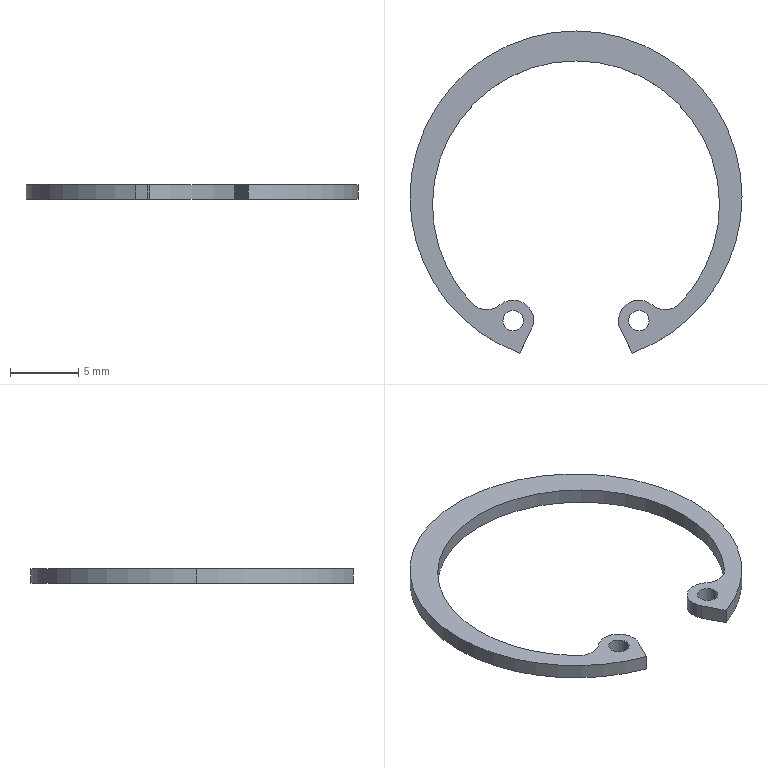Part | SolidWorks | features BaseBody 1 | 1 solid | 19 faces | box 24.35 x 23.625 x 1.1 mm | volume 130.198 mm3 | cylinder 15 | plane 4 | commonest cylinder face diameters 3 x5 1.5 x4 21.05 x3 24.35 x3
STEP:
#1=CARTESIAN_POINT('',(-5.362,-20.07,0.));
#2=VERTEX_POINT('',#1);
#3=CARTESIAN_POINT('',(-3.862,-20.07,0.));
#4=VERTEX_POINT('',#3);
#5=CARTESIAN_POINT('',(-4.612,-20.07,0.));
#6=DIRECTION('',(0.,0.,1.));
#7=DIRECTION('',(1.,0.,0.));
#8=AXIS2_PLACEMENT_3D('',#5,#6,#7);
#9=CIRCLE('',#8,0.75);
#10=EDGE_CURVE('',#2,#4,#9,.T.);
#11=ORIENTED_EDGE('',*,*,#10,.F.);
#12=CARTESIAN_POINT('',(-5.362,-20.07,1.1));
#13=VERTEX_POINT('',#12);
#14=CARTESIAN_POINT('',(-5.362,-20.07,0.));
#15=DIRECTION('',(0.,0.,1.));
#16=VECTOR('',#15,1000.);
#17=LINE('',#14,#16);
#18=EDGE_CURVE('',#2,#13,#17,.T.);
#19=ORIENTED_EDGE('',*,*,#18,.T.);
#20=CARTESIAN_POINT('',(-3.862,-20.07,1.1));
#21=VERTEX_POINT('',#20);
#22=CARTESIAN_POINT('',(-4.612,-20.07,1.1));
#23=DIRECTION('',(0.,0.,-1.));
#24=DIRECTION('',(1.,0.,0.));
#25=AXIS2_PLACEMENT_3D('',#22,#23,#24);
#26=CIRCLE('',#25,0.75);
#27=EDGE_CURVE('',#21,#13,#26,.T.);
#28=ORIENTED_EDGE('',*,*,#27,.F.);
#29=CARTESIAN_POINT('',(-3.862,-20.07,0.));
#30=DIRECTION('',(0.,0.,1.));
#31=VECTOR('',#30,1000.);
#32=LINE('',#29,#31);
#33=EDGE_CURVE('',#4,#21,#32,.T.);
#34=ORIENTED_EDGE('',*,*,#33,.F.);
#35=EDGE_LOOP('',(#11,#19,#28,#34));
#36=FACE_OUTER_BOUND('',#35,.T.);
#37=CARTESIAN_POINT('',(-4.612,-20.07,0.));
#38=DIRECTION('',(0.,0.,1.));
#39=DIRECTION('',(1.,0.,0.));
#40=AXIS2_PLACEMENT_3D('',#37,#38,#39);
#41=CYLINDRICAL_SURFACE('',#40,0.75);
#42=ADVANCED_FACE('',(#36),#41,.F.);
#43=CARTESIAN_POINT('',(3.862,-20.07,0.));
#44=VERTEX_POINT('',#43);
#45=CARTESIAN_POINT('',(5.362,-20.07,0.));
#46=VERTEX_POINT('',#45);
#47=CARTESIAN_POINT('',(4.612,-20.07,0.));
#48=DIRECTION('',(0.,0.,1.));
#49=DIRECTION('',(1.,0.,0.));
#50=AXIS2_PLACEMENT_3D('',#47,#48,#49);
#51=CIRCLE('',#50,0.75);
#52=EDGE_CURVE('',#44,#46,#51,.T.);
#53=ORIENTED_EDGE('',*,*,#52,.F.);
#54=CARTESIAN_POINT('',(3.862,-20.07,1.1));
#55=VERTEX_POINT('',#54);
#56=CARTESIAN_POINT('',(3.862,-20.07,0.));
#57=DIRECTION('',(0.,0.,1.));
#58=VECTOR('',#57,1000.);
#59=LINE('',#56,#58);
#60=EDGE_CURVE('',#44,#55,#59,.T.);
#61=ORIENTED_EDGE('',*,*,#60,.T.);
#62=CARTESIAN_POINT('',(5.362,-20.07,1.1));
#63=VERTEX_POINT('',#62);
#64=CARTESIAN_POINT('',(4.612,-20.07,1.1));
#65=DIRECTION('',(0.,0.,-1.));
#66=DIRECTION('',(1.,0.,0.));
#67=AXIS2_PLACEMENT_3D('',#64,#65,#66);
#68=CIRCLE('',#67,0.75);
#69=EDGE_CURVE('',#63,#55,#68,.T.);
#70=ORIENTED_EDGE('',*,*,#69,.F.);
#71=CARTESIAN_POINT('',(5.362,-20.07,0.));
#72=DIRECTION('',(0.,0.,1.));
#73=VECTOR('',#72,1000.);
#74=LINE('',#71,#73);
#75=EDGE_CURVE('',#46,#63,#74,.T.);
#76=ORIENTED_EDGE('',*,*,#75,.F.);
#77=EDGE_LOOP('',(#53,#61,#70,#76));
#78=FACE_OUTER_BOUND('',#77,.T.);
#79=CARTESIAN_POINT('',(4.612,-20.07,0.));
#80=DIRECTION('',(0.,0.,1.));
#81=DIRECTION('',(1.,0.,0.));
#82=AXIS2_PLACEMENT_3D('',#79,#80,#81);
#83=CYLINDRICAL_SURFACE('',#82,0.75);
#84=ADVANCED_FACE('',(#78),#83,.F.);
#85=CARTESIAN_POINT('',(-3.275,-20.75,0.));
#86=VERTEX_POINT('',#85);
#87=CARTESIAN_POINT('',(-3.112,-20.07,0.));
#88=VERTEX_POINT('',#87);
#89=CARTESIAN_POINT('',(-4.612,-20.07,0.));
#90=DIRECTION('',(0.,0.,1.));
#91=DIRECTION('',(1.,0.,0.));
#92=AXIS2_PLACEMENT_3D('',#89,#90,#91);
#93=CIRCLE('',#92,1.5);
#94=EDGE_CURVE('',#86,#88,#93,.T.);
#95=ORIENTED_EDGE('',*,*,#94,.T.);
#96=CARTESIAN_POINT('',(-3.112,-20.07,1.1));
#97=VERTEX_POINT('',#96);
#98=CARTESIAN_POINT('',(-3.112,-20.07,0.));
#99=DIRECTION('',(0.,0.,1.));
#100=VECTOR('',#99,1000.);
#101=LINE('',#98,#100);
#102=EDGE_CURVE('',#88,#97,#101,.T.);
#103=ORIENTED_EDGE('',*,*,#102,.T.);
#104=CARTESIAN_POINT('',(-3.275,-20.75,1.1));
#105=VERTEX_POINT('',#104);
#106=CARTESIAN_POINT('',(-4.612,-20.07,1.1));
#107=DIRECTION('',(0.,0.,1.));
#108=DIRECTION('',(1.,0.,0.));
#109=AXIS2_PLACEMENT_3D('',#106,#107,#108);
#110=CIRCLE('',#109,1.5);
#111=EDGE_CURVE('',#105,#97,#110,.T.);
#112=ORIENTED_EDGE('',*,*,#111,.F.);
#113=CARTESIAN_POINT('',(-3.275,-20.75,0.));
#114=DIRECTION('',(0.,0.,-1.));
#115=VECTOR('',#114,1000.);
#116=LINE('',#113,#115);
#117=EDGE_CURVE('',#105,#86,#116,.T.);
#118=ORIENTED_EDGE('',*,*,#117,.T.);
#119=EDGE_LOOP('',(#95,#103,#112,#118));
#120=FACE_OUTER_BOUND('',#119,.T.);
#121=CARTESIAN_POINT('',(-4.612,-20.07,0.));
#122=DIRECTION('',(0.,0.,1.));
#123=DIRECTION('',(1.,0.,0.));
#124=AXIS2_PLACEMENT_3D('',#121,#122,#123);
#125=CYLINDRICAL_SURFACE('',#124,1.5);
#126=ADVANCED_FACE('',(#120),#125,.T.);
#127=CARTESIAN_POINT('',(12.175,-11.,0.));
#128=VERTEX_POINT('',#127);
#129=CARTESIAN_POINT('',(-12.175,-11.,0.));
#130=VERTEX_POINT('',#129);
#131=CARTESIAN_POINT('',(0.,-11.,0.));
#132=DIRECTION('',(0.,0.,1.));
#133=DIRECTION('',(1.,0.,0.));
#134=AXIS2_PLACEMENT_3D('',#131,#132,#133);
#135=CIRCLE('',#134,12.175);
#136=EDGE_CURVE('',#128,#130,#135,.T.);
#137=ORIENTED_EDGE('',*,*,#136,.T.);
#138=CARTESIAN_POINT('',(-12.175,-11.,1.1));
#139=VERTEX_POINT('',#138);
#140=CARTESIAN_POINT('',(-12.175,-11.,0.));
#141=DIRECTION('',(0.,0.,1.));
#142=VECTOR('',#141,1000.);
#143=LINE('',#140,#142);
#144=EDGE_CURVE('',#130,#139,#143,.T.);
#145=ORIENTED_EDGE('',*,*,#144,.T.);
#146=CARTESIAN_POINT('',(12.175,-11.,1.1));
#147=VERTEX_POINT('',#146);
#148=CARTESIAN_POINT('',(0.,-11.,1.1));
#149=DIRECTION('',(0.,0.,1.));
#150=DIRECTION('',(1.,0.,0.));
#151=AXIS2_PLACEMENT_3D('',#148,#149,#150);
#152=CIRCLE('',#151,12.175);
#153=EDGE_CURVE('',#147,#139,#152,.T.);
#154=ORIENTED_EDGE('',*,*,#153,.F.);
#155=CARTESIAN_POINT('',(12.175,-11.,0.));
#156=DIRECTION('',(0.,0.,1.));
#157=VECTOR('',#156,1000.);
#158=LINE('',#155,#157);
#159=EDGE_CURVE('',#128,#147,#158,.T.);
#160=ORIENTED_EDGE('',*,*,#159,.F.);
#161=EDGE_LOOP('',(#137,#145,#154,#160));
#162=FACE_OUTER_BOUND('',#161,.T.);
#163=CARTESIAN_POINT('',(0.,-11.,0.));
#164=DIRECTION('',(0.,0.,1.));
#165=DIRECTION('',(1.,0.,0.));
#166=AXIS2_PLACEMENT_3D('',#163,#164,#165);
#167=CYLINDRICAL_SURFACE('',#166,12.175);
#168=ADVANCED_FACE('',(#162),#167,.T.);
#169=CARTESIAN_POINT('',(4.139,-22.45,0.));
#170=VERTEX_POINT('',#169);
#171=CARTESIAN_POINT('',(0.,-11.,0.));
#172=DIRECTION('',(0.,0.,1.));
#173=DIRECTION('',(1.,0.,0.));
#174=AXIS2_PLACEMENT_3D('',#171,#172,#173);
#175=CIRCLE('',#174,12.175);
#176=EDGE_CURVE('',#170,#128,#175,.T.);
#177=ORIENTED_EDGE('',*,*,#176,.T.);
#178=ORIENTED_EDGE('',*,*,#159,.T.);
#179=CARTESIAN_POINT('',(4.139,-22.45,1.1));
#180=VERTEX_POINT('',#179);
#181=CARTESIAN_POINT('',(0.,-11.,1.1));
#182=DIRECTION('',(0.,0.,1.));
#183=DIRECTION('',(1.,0.,0.));
#184=AXIS2_PLACEMENT_3D('',#181,#182,#183);
#185=CIRCLE('',#184,12.175);
#186=EDGE_CURVE('',#180,#147,#185,.T.);
#187=ORIENTED_EDGE('',*,*,#186,.F.);
#188=CARTESIAN_POINT('',(4.139,-22.45,0.));
#189=DIRECTION('',(0.,0.,-1.));
#190=VECTOR('',#189,1000.);
#191=LINE('',#188,#190);
#192=EDGE_CURVE('',#180,#170,#191,.T.);
#193=ORIENTED_EDGE('',*,*,#192,.T.);
#194=EDGE_LOOP('',(#177,#178,#187,#193));
#195=FACE_OUTER_BOUND('',#194,.T.);
#196=CARTESIAN_POINT('',(0.,-11.,0.));
#197=DIRECTION('',(0.,0.,1.));
#198=DIRECTION('',(1.,0.,0.));
#199=AXIS2_PLACEMENT_3D('',#196,#197,#198);
#200=CYLINDRICAL_SURFACE('',#199,12.175);
#201=ADVANCED_FACE('',(#195),#200,.T.);
#202=CARTESIAN_POINT('',(-10.525,-11.55,0.));
#203=VERTEX_POINT('',#202);
#204=CARTESIAN_POINT('',(-7.626,-18.804,0.));
#205=VERTEX_POINT('',#204);
#206=CARTESIAN_POINT('',(0.,-11.55,0.));
#207=DIRECTION('',(0.,0.,1.));
#208=DIRECTION('',(1.,0.,0.));
#209=AXIS2_PLACEMENT_3D('',#206,#207,#208);
#210=CIRCLE('',#209,10.525);
#211=EDGE_CURVE('',#203,#205,#210,.T.);
#212=ORIENTED_EDGE('',*,*,#211,.F.);
#213=CARTESIAN_POINT('',(-10.525,-11.55,1.1));
#214=VERTEX_POINT('',#213);
#215=CARTESIAN_POINT('',(-10.525,-11.55,0.));
#216=DIRECTION('',(0.,0.,1.));
#217=VECTOR('',#216,1000.);
#218=LINE('',#215,#217);
#219=EDGE_CURVE('',#203,#214,#218,.T.);
#220=ORIENTED_EDGE('',*,*,#219,.T.);
#221=CARTESIAN_POINT('',(-7.626,-18.804,1.1));
#222=VERTEX_POINT('',#221);
#223=CARTESIAN_POINT('',(0.,-11.55,1.1));
#224=DIRECTION('',(0.,0.,-1.));
#225=DIRECTION('',(1.,0.,0.));
#226=AXIS2_PLACEMENT_3D('',#223,#224,#225);
#227=CIRCLE('',#226,10.525);
#228=EDGE_CURVE('',#222,#214,#227,.T.);
#229=ORIENTED_EDGE('',*,*,#228,.F.);
#230=CARTESIAN_POINT('',(-7.626,-18.804,0.));
#231=DIRECTION('',(0.,0.,-1.));
#232=VECTOR('',#231,1000.);
#233=LINE('',#230,#232);
#234=EDGE_CURVE('',#222,#205,#233,.T.);
#235=ORIENTED_EDGE('',*,*,#234,.T.);
#236=EDGE_LOOP('',(#212,#220,#229,#235));
#237=FACE_OUTER_BOUND('',#236,.T.);
#238=CARTESIAN_POINT('',(0.,-11.55,0.));
#239=DIRECTION('',(0.,0.,1.));
#240=DIRECTION('',(1.,0.,0.));
#241=AXIS2_PLACEMENT_3D('',#238,#239,#240);
#242=CYLINDRICAL_SURFACE('',#241,10.525);
#243=ADVANCED_FACE('',(#237),#242,.F.);
#244=ORIENTED_EDGE('',*,*,#219,.F.);
#245=CARTESIAN_POINT('',(10.525,-11.55,0.));
#246=VERTEX_POINT('',#245);
#247=CARTESIAN_POINT('',(0.,-11.55,0.));
#248=DIRECTION('',(0.,0.,1.));
#249=DIRECTION('',(1.,0.,0.));
#250=AXIS2_PLACEMENT_3D('',#247,#248,#249);
#251=CIRCLE('',#250,10.525);
#252=EDGE_CURVE('',#246,#203,#251,.T.);
#253=ORIENTED_EDGE('',*,*,#252,.F.);
#254=CARTESIAN_POINT('',(10.525,-11.55,1.1));
#255=VERTEX_POINT('',#254);
#256=CARTESIAN_POINT('',(10.525,-11.55,0.));
#257=DIRECTION('',(0.,0.,1.));
#258=VECTOR('',#257,1000.);
#259=LINE('',#256,#258);
#260=EDGE_CURVE('',#246,#255,#259,.T.);
#261=ORIENTED_EDGE('',*,*,#260,.T.);
#262=CARTESIAN_POINT('',(0.,-11.55,1.1));
#263=DIRECTION('',(0.,0.,-1.));
#264=DIRECTION('',(1.,0.,0.));
#265=AXIS2_PLACEMENT_3D('',#262,#263,#264);
#266=CIRCLE('',#265,10.525);
#267=EDGE_CURVE('',#214,#255,#266,.T.);
#268=ORIENTED_EDGE('',*,*,#267,.F.);
#269=EDGE_LOOP('',(#244,#253,#261,#268));
#270=FACE_OUTER_BOUND('',#269,.T.);
#271=CARTESIAN_POINT('',(0.,-11.55,0.));
#272=DIRECTION('',(0.,0.,1.));
#273=DIRECTION('',(1.,0.,0.));
#274=AXIS2_PLACEMENT_3D('',#271,#272,#273);
#275=CYLINDRICAL_SURFACE('',#274,10.525);
#276=ADVANCED_FACE('',(#270),#275,.F.);
#277=ORIENTED_EDGE('',*,*,#27,.T.);
#278=CARTESIAN_POINT('',(-4.612,-20.07,1.1));
#279=DIRECTION('',(0.,0.,-1.));
#280=DIRECTION('',(1.,0.,0.));
#281=AXIS2_PLACEMENT_3D('',#278,#279,#280);
#282=CIRCLE('',#281,0.75);
#283=EDGE_CURVE('',#13,#21,#282,.T.);
#284=ORIENTED_EDGE('',*,*,#283,.T.);
#285=EDGE_LOOP('',(#277,#284));
#286=FACE_BOUND('',#285,.T.);
#287=ORIENTED_EDGE('',*,*,#69,.T.);
#288=CARTESIAN_POINT('',(4.612,-20.07,1.1));
#289=DIRECTION('',(0.,0.,-1.));
#290=DIRECTION('',(1.,0.,0.));
#291=AXIS2_PLACEMENT_3D('',#288,#289,#290);
#292=CIRCLE('',#291,0.75);
#293=EDGE_CURVE('',#55,#63,#292,.T.);
#294=ORIENTED_EDGE('',*,*,#293,.T.);
#295=EDGE_LOOP('',(#287,#294));
#296=FACE_BOUND('',#295,.T.);
#297=ORIENTED_EDGE('',*,*,#111,.T.);
#298=CARTESIAN_POINT('',(-5.576,-18.92,1.1));
#299=VERTEX_POINT('',#298);
#300=CARTESIAN_POINT('',(-4.612,-20.07,1.1));
#301=DIRECTION('',(0.,0.,1.));
#302=DIRECTION('',(1.,0.,0.));
#303=AXIS2_PLACEMENT_3D('',#300,#301,#302);
#304=CIRCLE('',#303,1.5);
#305=EDGE_CURVE('',#97,#299,#304,.T.);
#306=ORIENTED_EDGE('',*,*,#305,.T.);
#307=CARTESIAN_POINT('',(-6.539,-17.77,1.1));
#308=DIRECTION('',(0.,0.,-1.));
#309=DIRECTION('',(1.,0.,0.));
#310=AXIS2_PLACEMENT_3D('',#307,#308,#309);
#311=CIRCLE('',#310,1.5);
#312=EDGE_CURVE('',#299,#222,#311,.T.);
#313=ORIENTED_EDGE('',*,*,#312,.T.);
#314=ORIENTED_EDGE('',*,*,#228,.T.);
#315=ORIENTED_EDGE('',*,*,#267,.T.);
#316=CARTESIAN_POINT('',(7.626,-18.804,1.1));
#317=VERTEX_POINT('',#316);
#318=CARTESIAN_POINT('',(0.,-11.55,1.1));
#319=DIRECTION('',(0.,0.,-1.));
#320=DIRECTION('',(1.,0.,0.));
#321=AXIS2_PLACEMENT_3D('',#318,#319,#320);
#322=CIRCLE('',#321,10.525);
#323=EDGE_CURVE('',#255,#317,#322,.T.);
#324=ORIENTED_EDGE('',*,*,#323,.T.);
#325=CARTESIAN_POINT('',(5.576,-18.92,1.1));
#326=VERTEX_POINT('',#325);
#327=CARTESIAN_POINT('',(6.539,-17.77,1.1));
#328=DIRECTION('',(0.,0.,-1.));
#329=DIRECTION('',(1.,0.,0.));
#330=AXIS2_PLACEMENT_3D('',#327,#328,#329);
#331=CIRCLE('',#330,1.5);
#332=EDGE_CURVE('',#317,#326,#331,.T.);
#333=ORIENTED_EDGE('',*,*,#332,.T.);
#334=CARTESIAN_POINT('',(3.275,-20.75,1.1));
#335=VERTEX_POINT('',#334);
#336=CARTESIAN_POINT('',(4.612,-20.07,1.1));
#337=DIRECTION('',(0.,0.,1.));
#338=DIRECTION('',(1.,0.,0.));
#339=AXIS2_PLACEMENT_3D('',#336,#337,#338);
#340=CIRCLE('',#339,1.5);
#341=EDGE_CURVE('',#326,#335,#340,.T.);
#342=ORIENTED_EDGE('',*,*,#341,.T.);
#343=CARTESIAN_POINT('',(3.275,-20.75,1.1));
#344=DIRECTION('',(0.4533,-0.8914,0.));
#345=VECTOR('',#344,1000.);
#346=LINE('',#343,#345);
#347=EDGE_CURVE('',#335,#180,#346,.T.);
#348=ORIENTED_EDGE('',*,*,#347,.T.);
#349=ORIENTED_EDGE('',*,*,#186,.T.);
#350=ORIENTED_EDGE('',*,*,#153,.T.);
#351=CARTESIAN_POINT('',(-4.14,-22.45,1.1));
#352=VERTEX_POINT('',#351);
#353=CARTESIAN_POINT('',(0.,-11.,1.1));
#354=DIRECTION('',(0.,0.,1.));
#355=DIRECTION('',(1.,0.,0.));
#356=AXIS2_PLACEMENT_3D('',#353,#354,#355);
#357=CIRCLE('',#356,12.175);
#358=EDGE_CURVE('',#139,#352,#357,.T.);
#359=ORIENTED_EDGE('',*,*,#358,.T.);
#360=CARTESIAN_POINT('',(-4.14,-22.45,1.1));
#361=DIRECTION('',(0.4533,0.8914,0.));
#362=VECTOR('',#361,1000.);
#363=LINE('',#360,#362);
#364=EDGE_CURVE('',#352,#105,#363,.T.);
#365=ORIENTED_EDGE('',*,*,#364,.T.);
#366=EDGE_LOOP('',(#297,#306,#313,#314,#315,#324,#333,#342,#348,#349,#350,#359,#365));
#367=FACE_OUTER_BOUND('',#366,.T.);
#368=CARTESIAN_POINT('',(-0.03738,-10.997,1.1));
#369=DIRECTION('',(0.,0.,1.));
#370=DIRECTION('',(1.,0.,0.));
#371=AXIS2_PLACEMENT_3D('',#368,#369,#370);
#372=PLANE('',#371);
#373=ADVANCED_FACE('',(#286,#296,#367),#372,.T.);
#374=ORIENTED_EDGE('',*,*,#18,.F.);
#375=CARTESIAN_POINT('',(-4.612,-20.07,0.));
#376=DIRECTION('',(0.,0.,1.));
#377=DIRECTION('',(1.,0.,0.));
#378=AXIS2_PLACEMENT_3D('',#375,#376,#377);
#379=CIRCLE('',#378,0.75);
#380=EDGE_CURVE('',#4,#2,#379,.T.);
#381=ORIENTED_EDGE('',*,*,#380,.F.);
#382=ORIENTED_EDGE('',*,*,#33,.T.);
#383=ORIENTED_EDGE('',*,*,#283,.F.);
#384=EDGE_LOOP('',(#374,#381,#382,#383));
#385=FACE_OUTER_BOUND('',#384,.T.);
#386=CARTESIAN_POINT('',(-4.612,-20.07,0.));
#387=DIRECTION('',(0.,0.,1.));
#388=DIRECTION('',(1.,0.,0.));
#389=AXIS2_PLACEMENT_3D('',#386,#387,#388);
#390=CYLINDRICAL_SURFACE('',#389,0.75);
#391=ADVANCED_FACE('',(#385),#390,.F.);
#392=ORIENTED_EDGE('',*,*,#60,.F.);
#393=CARTESIAN_POINT('',(4.612,-20.07,0.));
#394=DIRECTION('',(0.,0.,1.));
#395=DIRECTION('',(1.,0.,0.));
#396=AXIS2_PLACEMENT_3D('',#393,#394,#395);
#397=CIRCLE('',#396,0.75);
#398=EDGE_CURVE('',#46,#44,#397,.T.);
#399=ORIENTED_EDGE('',*,*,#398,.F.);
#400=ORIENTED_EDGE('',*,*,#75,.T.);
#401=ORIENTED_EDGE('',*,*,#293,.F.);
#402=EDGE_LOOP('',(#392,#399,#400,#401));
#403=FACE_OUTER_BOUND('',#402,.T.);
#404=CARTESIAN_POINT('',(4.612,-20.07,0.));
#405=DIRECTION('',(0.,0.,1.));
#406=DIRECTION('',(1.,0.,0.));
#407=AXIS2_PLACEMENT_3D('',#404,#405,#406);
#408=CYLINDRICAL_SURFACE('',#407,0.75);
#409=ADVANCED_FACE('',(#403),#408,.F.);
#410=CARTESIAN_POINT('',(-5.576,-18.92,0.));
#411=VERTEX_POINT('',#410);
#412=CARTESIAN_POINT('',(-5.576,-18.92,0.));
#413=DIRECTION('',(0.,0.,1.));
#414=VECTOR('',#413,1000.);
#415=LINE('',#412,#414);
#416=EDGE_CURVE('',#411,#299,#415,.T.);
#417=ORIENTED_EDGE('',*,*,#416,.F.);
#418=CARTESIAN_POINT('',(-6.539,-17.77,0.));
#419=DIRECTION('',(0.,0.,1.));
#420=DIRECTION('',(1.,0.,0.));
#421=AXIS2_PLACEMENT_3D('',#418,#419,#420);
#422=CIRCLE('',#421,1.5);
#423=EDGE_CURVE('',#205,#411,#422,.T.);
#424=ORIENTED_EDGE('',*,*,#423,.F.);
#425=ORIENTED_EDGE('',*,*,#234,.F.);
#426=ORIENTED_EDGE('',*,*,#312,.F.);
#427=EDGE_LOOP('',(#417,#424,#425,#426));
#428=FACE_OUTER_BOUND('',#427,.T.);
#429=CARTESIAN_POINT('',(-6.539,-17.77,0.));
#430=DIRECTION('',(0.,0.,1.));
#431=DIRECTION('',(1.,0.,0.));
#432=AXIS2_PLACEMENT_3D('',#429,#430,#431);
#433=CYLINDRICAL_SURFACE('',#432,1.5);
#434=ADVANCED_FACE('',(#428),#433,.F.);
#435=ORIENTED_EDGE('',*,*,#102,.F.);
#436=CARTESIAN_POINT('',(-4.612,-20.07,0.));
#437=DIRECTION('',(0.,0.,1.));
#438=DIRECTION('',(1.,0.,0.));
#439=AXIS2_PLACEMENT_3D('',#436,#437,#438);
#440=CIRCLE('',#439,1.5);
#441=EDGE_CURVE('',#88,#411,#440,.T.);
#442=ORIENTED_EDGE('',*,*,#441,.T.);
#443=ORIENTED_EDGE('',*,*,#416,.T.);
#444=ORIENTED_EDGE('',*,*,#305,.F.);
#445=EDGE_LOOP('',(#435,#442,#443,#444));
#446=FACE_OUTER_BOUND('',#445,.T.);
#447=CARTESIAN_POINT('',(-4.612,-20.07,0.));
#448=DIRECTION('',(0.,0.,1.));
#449=DIRECTION('',(1.,0.,0.));
#450=AXIS2_PLACEMENT_3D('',#447,#448,#449);
#451=CYLINDRICAL_SURFACE('',#450,1.5);
#452=ADVANCED_FACE('',(#446),#451,.T.);
#453=CARTESIAN_POINT('',(-4.14,-22.45,0.));
#454=VERTEX_POINT('',#453);
#455=CARTESIAN_POINT('',(-3.275,-20.75,0.));
#456=DIRECTION('',(0.4533,0.8914,0.));
#457=VECTOR('',#456,1000.);
#458=LINE('',#455,#457);
#459=EDGE_CURVE('',#454,#86,#458,.T.);
#460=ORIENTED_EDGE('',*,*,#459,.T.);
#461=ORIENTED_EDGE('',*,*,#117,.F.);
#462=ORIENTED_EDGE('',*,*,#364,.F.);
#463=CARTESIAN_POINT('',(-4.14,-22.45,0.));
#464=DIRECTION('',(0.,0.,-1.));
#465=VECTOR('',#464,1000.);
#466=LINE('',#463,#465);
#467=EDGE_CURVE('',#352,#454,#466,.T.);
#468=ORIENTED_EDGE('',*,*,#467,.T.);
#469=EDGE_LOOP('',(#460,#461,#462,#468));
#470=FACE_OUTER_BOUND('',#469,.T.);
#471=CARTESIAN_POINT('',(-3.275,-20.75,0.));
#472=DIRECTION('',(0.8914,-0.4533,0.));
#473=DIRECTION('',(0.4533,0.8914,0.));
#474=AXIS2_PLACEMENT_3D('',#471,#472,#473);
#475=PLANE('',#474);
#476=ADVANCED_FACE('',(#470),#475,.T.);
#477=ORIENTED_EDGE('',*,*,#144,.F.);
#478=CARTESIAN_POINT('',(0.,-11.,0.));
#479=DIRECTION('',(0.,0.,1.));
#480=DIRECTION('',(1.,0.,0.));
#481=AXIS2_PLACEMENT_3D('',#478,#479,#480);
#482=CIRCLE('',#481,12.175);
#483=EDGE_CURVE('',#130,#454,#482,.T.);
#484=ORIENTED_EDGE('',*,*,#483,.T.);
#485=ORIENTED_EDGE('',*,*,#467,.F.);
#486=ORIENTED_EDGE('',*,*,#358,.F.);
#487=EDGE_LOOP('',(#477,#484,#485,#486));
#488=FACE_OUTER_BOUND('',#487,.T.);
#489=CARTESIAN_POINT('',(0.,-11.,0.));
#490=DIRECTION('',(0.,0.,1.));
#491=DIRECTION('',(1.,0.,0.));
#492=AXIS2_PLACEMENT_3D('',#489,#490,#491);
#493=CYLINDRICAL_SURFACE('',#492,12.175);
#494=ADVANCED_FACE('',(#488),#493,.T.);
#495=CARTESIAN_POINT('',(3.275,-20.75,0.));
#496=VERTEX_POINT('',#495);
#497=CARTESIAN_POINT('',(4.14,-22.45,0.));
#498=DIRECTION('',(0.4533,-0.8914,0.));
#499=VECTOR('',#498,1000.);
#500=LINE('',#497,#499);
#501=EDGE_CURVE('',#496,#170,#500,.T.);
#502=ORIENTED_EDGE('',*,*,#501,.T.);
#503=ORIENTED_EDGE('',*,*,#192,.F.);
#504=ORIENTED_EDGE('',*,*,#347,.F.);
#505=CARTESIAN_POINT('',(3.275,-20.75,0.));
#506=DIRECTION('',(0.,0.,-1.));
#507=VECTOR('',#506,1000.);
#508=LINE('',#505,#507);
#509=EDGE_CURVE('',#335,#496,#508,.T.);
#510=ORIENTED_EDGE('',*,*,#509,.T.);
#511=EDGE_LOOP('',(#502,#503,#504,#510));
#512=FACE_OUTER_BOUND('',#511,.T.);
#513=CARTESIAN_POINT('',(4.14,-22.45,0.));
#514=DIRECTION('',(-0.8914,-0.4533,0.));
#515=DIRECTION('',(0.4533,-0.8914,0.));
#516=AXIS2_PLACEMENT_3D('',#513,#514,#515);
#517=PLANE('',#516);
#518=ADVANCED_FACE('',(#512),#517,.T.);
#519=CARTESIAN_POINT('',(5.576,-18.92,0.));
#520=VERTEX_POINT('',#519);
#521=CARTESIAN_POINT('',(4.612,-20.07,0.));
#522=DIRECTION('',(0.,0.,1.));
#523=DIRECTION('',(1.,0.,0.));
#524=AXIS2_PLACEMENT_3D('',#521,#522,#523);
#525=CIRCLE('',#524,1.5);
#526=EDGE_CURVE('',#520,#496,#525,.T.);
#527=ORIENTED_EDGE('',*,*,#526,.T.);
#528=ORIENTED_EDGE('',*,*,#509,.F.);
#529=ORIENTED_EDGE('',*,*,#341,.F.);
#530=CARTESIAN_POINT('',(5.576,-18.92,0.));
#531=DIRECTION('',(0.,0.,-1.));
#532=VECTOR('',#531,1000.);
#533=LINE('',#530,#532);
#534=EDGE_CURVE('',#326,#520,#533,.T.);
#535=ORIENTED_EDGE('',*,*,#534,.T.);
#536=EDGE_LOOP('',(#527,#528,#529,#535));
#537=FACE_OUTER_BOUND('',#536,.T.);
#538=CARTESIAN_POINT('',(4.612,-20.07,0.));
#539=DIRECTION('',(0.,0.,1.));
#540=DIRECTION('',(1.,0.,0.));
#541=AXIS2_PLACEMENT_3D('',#538,#539,#540);
#542=CYLINDRICAL_SURFACE('',#541,1.5);
#543=ADVANCED_FACE('',(#537),#542,.T.);
#544=CARTESIAN_POINT('',(7.626,-18.804,0.));
#545=VERTEX_POINT('',#544);
#546=CARTESIAN_POINT('',(7.626,-18.804,0.));
#547=DIRECTION('',(0.,0.,1.));
#548=VECTOR('',#547,1000.);
#549=LINE('',#546,#548);
#550=EDGE_CURVE('',#545,#317,#549,.T.);
#551=ORIENTED_EDGE('',*,*,#550,.F.);
#552=CARTESIAN_POINT('',(6.539,-17.77,0.));
#553=DIRECTION('',(0.,0.,1.));
#554=DIRECTION('',(1.,0.,0.));
#555=AXIS2_PLACEMENT_3D('',#552,#553,#554);
#556=CIRCLE('',#555,1.5);
#557=EDGE_CURVE('',#520,#545,#556,.T.);
#558=ORIENTED_EDGE('',*,*,#557,.F.);
#559=ORIENTED_EDGE('',*,*,#534,.F.);
#560=ORIENTED_EDGE('',*,*,#332,.F.);
#561=EDGE_LOOP('',(#551,#558,#559,#560));
#562=FACE_OUTER_BOUND('',#561,.T.);
#563=CARTESIAN_POINT('',(6.539,-17.77,0.));
#564=DIRECTION('',(0.,0.,1.));
#565=DIRECTION('',(1.,0.,0.));
#566=AXIS2_PLACEMENT_3D('',#563,#564,#565);
#567=CYLINDRICAL_SURFACE('',#566,1.5);
#568=ADVANCED_FACE('',(#562),#567,.F.);
#569=ORIENTED_EDGE('',*,*,#260,.F.);
#570=CARTESIAN_POINT('',(0.,-11.55,0.));
#571=DIRECTION('',(0.,0.,1.));
#572=DIRECTION('',(1.,0.,0.));
#573=AXIS2_PLACEMENT_3D('',#570,#571,#572);
#574=CIRCLE('',#573,10.525);
#575=EDGE_CURVE('',#545,#246,#574,.T.);
#576=ORIENTED_EDGE('',*,*,#575,.F.);
#577=ORIENTED_EDGE('',*,*,#550,.T.);
#578=ORIENTED_EDGE('',*,*,#323,.F.);
#579=EDGE_LOOP('',(#569,#576,#577,#578));
#580=FACE_OUTER_BOUND('',#579,.T.);
#581=CARTESIAN_POINT('',(0.,-11.55,0.));
#582=DIRECTION('',(0.,0.,1.));
#583=DIRECTION('',(1.,0.,0.));
#584=AXIS2_PLACEMENT_3D('',#581,#582,#583);
#585=CYLINDRICAL_SURFACE('',#584,10.525);
#586=ADVANCED_FACE('',(#580),#585,.F.);
#587=ORIENTED_EDGE('',*,*,#380,.T.);
#588=ORIENTED_EDGE('',*,*,#10,.T.);
#589=EDGE_LOOP('',(#587,#588));
#590=FACE_BOUND('',#589,.T.);
#591=ORIENTED_EDGE('',*,*,#398,.T.);
#592=ORIENTED_EDGE('',*,*,#52,.T.);
#593=EDGE_LOOP('',(#591,#592));
#594=FACE_BOUND('',#593,.T.);
#595=ORIENTED_EDGE('',*,*,#423,.T.);
#596=ORIENTED_EDGE('',*,*,#441,.F.);
#597=ORIENTED_EDGE('',*,*,#94,.F.);
#598=ORIENTED_EDGE('',*,*,#459,.F.);
#599=ORIENTED_EDGE('',*,*,#483,.F.);
#600=ORIENTED_EDGE('',*,*,#136,.F.);
#601=ORIENTED_EDGE('',*,*,#176,.F.);
#602=ORIENTED_EDGE('',*,*,#501,.F.);
#603=ORIENTED_EDGE('',*,*,#526,.F.);
#604=ORIENTED_EDGE('',*,*,#557,.T.);
#605=ORIENTED_EDGE('',*,*,#575,.T.);
#606=ORIENTED_EDGE('',*,*,#252,.T.);
#607=ORIENTED_EDGE('',*,*,#211,.T.);
#608=EDGE_LOOP('',(#595,#596,#597,#598,#599,#600,#601,#602,#603,#604,#605,#606,#607));
#609=FACE_OUTER_BOUND('',#608,.T.);
#610=CARTESIAN_POINT('',(-0.03738,-10.997,0.));
#611=DIRECTION('',(0.,0.,1.));
#612=DIRECTION('',(1.,0.,0.));
#613=AXIS2_PLACEMENT_3D('',#610,#611,#612);
#614=PLANE('',#613);
#615=ADVANCED_FACE('',(#590,#594,#609),#614,.F.);
#616=CLOSED_SHELL('',(#42,#84,#126,#168,#201,#243,#276,#373,#391,#409,#434,#452,#476,#494,#518,#543,#568,#586,#615));
#617=MANIFOLD_SOLID_BREP('',#616);
#618=CARTESIAN_POINT('',(0.,0.,0.));
#619=DIRECTION('',(0.,0.,1.));
#620=DIRECTION('',(1.,0.,0.));
#621=AXIS2_PLACEMENT_3D('',#618,#619,#620);
#622=(LENGTH_UNIT()NAMED_UNIT(*)SI_UNIT(.MILLI.,.METRE.));
#623=UNCERTAINTY_MEASURE_WITH_UNIT(LENGTH_MEASURE(0.00001),#622,'','');
#624=(NAMED_UNIT(*)PLANE_ANGLE_UNIT()SI_UNIT($,.RADIAN.));
#625=(NAMED_UNIT(*)SI_UNIT($,.STERADIAN.)SOLID_ANGLE_UNIT());
#626=(GEOMETRIC_REPRESENTATION_CONTEXT(3)GLOBAL_UNCERTAINTY_ASSIGNED_CONTEXT((#623))GLOBAL_UNIT_ASSIGNED_CONTEXT((#622,#624,#625))REPRESENTATION_CONTEXT('',''));
#627=ADVANCED_BREP_SHAPE_REPRESENTATION('',(#617,#621),#626);